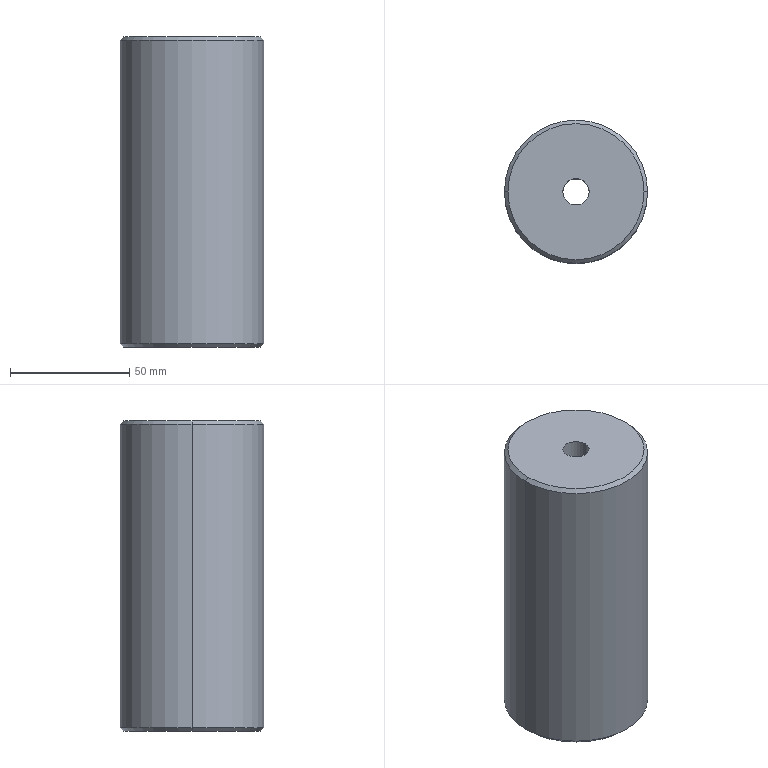Part | 1 solid | 13 faces | box 60 x 60 x 130 mm | volume 352156 mm3 | cylinder 6 | cone 4 | plane 3 | commonest cylinder face diameters 11 x2 17 x2 60 x2
STEP:
#1=CARTESIAN_POINT('',(0.,0.,0.));
#2=DIRECTION('',(0.,0.,1.));
#3=DIRECTION('',(1.,0.,0.));
#4=AXIS2_PLACEMENT_3D('',#1,#2,#3);
#5=CARTESIAN_POINT('',(24.,631.5,-191.551));
#6=VERTEX_POINT('',#5);
#7=CARTESIAN_POINT('',(24.,631.5,-64.551));
#8=VERTEX_POINT('',#7);
#9=CARTESIAN_POINT('',(24.,631.5,-191.551));
#10=DIRECTION('',(0.,0.,1.));
#11=VECTOR('',#10,1.);
#12=LINE('',#9,#11);
#13=CARTESIAN_POINT('',(-6.,631.5,-193.051));
#14=DIRECTION('',(0.,0.,1.));
#15=DIRECTION('',(0.,-1.,0.));
#16=AXIS2_PLACEMENT_3D('',#13,#14,#15);
#17=CYLINDRICAL_SURFACE('',#16,30.);
#18=CARTESIAN_POINT('',(1.571,1.5));
#19=DIRECTION('',(0.,1.));
#20=VECTOR('',#19,1.);
#21=LINE('',#18,#20);
#22=(GEOMETRIC_REPRESENTATION_CONTEXT(2)PARAMETRIC_REPRESENTATION_CONTEXT()REPRESENTATION_CONTEXT('',''));
#23=DEFINITIONAL_REPRESENTATION('',(#21),#22);
#24=PCURVE('',#17,#23);
#25=CARTESIAN_POINT('',(-6.,631.5,-193.051));
#26=DIRECTION('',(0.,0.,1.));
#27=DIRECTION('',(0.,1.,0.));
#28=AXIS2_PLACEMENT_3D('',#25,#26,#27);
#29=CYLINDRICAL_SURFACE('',#28,30.);
#30=CARTESIAN_POINT('',(4.712,1.5));
#31=DIRECTION('',(0.,1.));
#32=VECTOR('',#31,1.);
#33=LINE('',#30,#32);
#34=(GEOMETRIC_REPRESENTATION_CONTEXT(2)PARAMETRIC_REPRESENTATION_CONTEXT()REPRESENTATION_CONTEXT('',''));
#35=DEFINITIONAL_REPRESENTATION('',(#33),#34);
#36=PCURVE('',#29,#35);
#37=SURFACE_CURVE('',#12,(#24,#36),.PCURVE_S1.);
#38=EDGE_CURVE('',#6,#8,#37,.T.);
#39=ORIENTED_EDGE('',*,*,#38,.F.);
#40=CARTESIAN_POINT('',(-36.,631.5,-191.551));
#41=VERTEX_POINT('',#40);
#42=CARTESIAN_POINT('',(-6.,631.5,-191.551));
#43=DIRECTION('',(0.,0.,1.));
#44=DIRECTION('',(1.,0.,0.));
#45=AXIS2_PLACEMENT_3D('',#42,#43,#44);
#46=CIRCLE('',#45,30.);
#47=CARTESIAN_POINT('',(1.571,1.5));
#48=DIRECTION('',(1.,0.));
#49=VECTOR('',#48,1.);
#50=LINE('',#47,#49);
#51=(GEOMETRIC_REPRESENTATION_CONTEXT(2)PARAMETRIC_REPRESENTATION_CONTEXT()REPRESENTATION_CONTEXT('',''));
#52=DEFINITIONAL_REPRESENTATION('',(#50),#51);
#53=PCURVE('',#17,#52);
#54=CARTESIAN_POINT('',(-6.,631.5,-191.551));
#55=DIRECTION('',(0.,0.,1.));
#56=DIRECTION('',(0.,-1.,0.));
#57=AXIS2_PLACEMENT_3D('',#54,#55,#56);
#58=CONICAL_SURFACE('',#57,30.,0.7854);
#59=CARTESIAN_POINT('',(1.571,0.));
#60=DIRECTION('',(1.,0.));
#61=VECTOR('',#60,1.);
#62=LINE('',#59,#61);
#63=(GEOMETRIC_REPRESENTATION_CONTEXT(2)PARAMETRIC_REPRESENTATION_CONTEXT()REPRESENTATION_CONTEXT('',''));
#64=DEFINITIONAL_REPRESENTATION('',(#62),#63);
#65=PCURVE('',#58,#64);
#66=SURFACE_CURVE('',#46,(#53,#65),.PCURVE_S1.);
#67=EDGE_CURVE('',#6,#41,#66,.T.);
#68=ORIENTED_EDGE('',*,*,#67,.T.);
#69=CARTESIAN_POINT('',(-36.,631.5,-64.551));
#70=VERTEX_POINT('',#69);
#71=CARTESIAN_POINT('',(-36.,631.5,-191.551));
#72=DIRECTION('',(0.,0.,1.));
#73=VECTOR('',#72,1.);
#74=LINE('',#71,#73);
#75=CARTESIAN_POINT('',(4.712,1.5));
#76=DIRECTION('',(0.,1.));
#77=VECTOR('',#76,1.);
#78=LINE('',#75,#77);
#79=(GEOMETRIC_REPRESENTATION_CONTEXT(2)PARAMETRIC_REPRESENTATION_CONTEXT()REPRESENTATION_CONTEXT('',''));
#80=DEFINITIONAL_REPRESENTATION('',(#78),#79);
#81=PCURVE('',#17,#80);
#82=CARTESIAN_POINT('',(1.571,1.5));
#83=DIRECTION('',(0.,1.));
#84=VECTOR('',#83,1.);
#85=LINE('',#82,#84);
#86=(GEOMETRIC_REPRESENTATION_CONTEXT(2)PARAMETRIC_REPRESENTATION_CONTEXT()REPRESENTATION_CONTEXT('',''));
#87=DEFINITIONAL_REPRESENTATION('',(#85),#86);
#88=PCURVE('',#29,#87);
#89=SURFACE_CURVE('',#74,(#81,#88),.PCURVE_S1.);
#90=EDGE_CURVE('',#41,#70,#89,.T.);
#91=ORIENTED_EDGE('',*,*,#90,.T.);
#92=CARTESIAN_POINT('',(-6.,631.5,-64.551));
#93=DIRECTION('',(0.,0.,-1.));
#94=DIRECTION('',(-1.,0.,0.));
#95=AXIS2_PLACEMENT_3D('',#92,#93,#94);
#96=CIRCLE('',#95,30.);
#97=CARTESIAN_POINT('',(4.712,128.5));
#98=DIRECTION('',(-1.,0.));
#99=VECTOR('',#98,1.);
#100=LINE('',#97,#99);
#101=(GEOMETRIC_REPRESENTATION_CONTEXT(2)PARAMETRIC_REPRESENTATION_CONTEXT()REPRESENTATION_CONTEXT('',''));
#102=DEFINITIONAL_REPRESENTATION('',(#100),#101);
#103=PCURVE('',#17,#102);
#104=CARTESIAN_POINT('',(-6.,631.5,-63.051));
#105=DIRECTION('',(0.,0.,-1.));
#106=DIRECTION('',(0.,-1.,0.));
#107=AXIS2_PLACEMENT_3D('',#104,#105,#106);
#108=CONICAL_SURFACE('',#107,28.5,0.7854);
#109=CARTESIAN_POINT('',(1.571,1.5));
#110=DIRECTION('',(1.,0.));
#111=VECTOR('',#110,1.);
#112=LINE('',#109,#111);
#113=(GEOMETRIC_REPRESENTATION_CONTEXT(2)PARAMETRIC_REPRESENTATION_CONTEXT()REPRESENTATION_CONTEXT('',''));
#114=DEFINITIONAL_REPRESENTATION('',(#112),#113);
#115=PCURVE('',#108,#114);
#116=SURFACE_CURVE('',#96,(#103,#115),.PCURVE_S1.);
#117=EDGE_CURVE('',#70,#8,#116,.T.);
#118=ORIENTED_EDGE('',*,*,#117,.T.);
#119=EDGE_LOOP('',(#39,#68,#91,#118));
#120=FACE_BOUND('',#119,.T.);
#121=ADVANCED_FACE('',(#120),#17,.T.);
#122=CARTESIAN_POINT('',(-34.5,631.5,-193.051));
#123=VERTEX_POINT('',#122);
#124=CARTESIAN_POINT('',(-34.5,631.5,-193.051));
#125=DIRECTION('',(-0.7071,0.,0.7071));
#126=VECTOR('',#125,1.);
#127=LINE('',#124,#126);
#128=CARTESIAN_POINT('',(-6.,631.5,-191.551));
#129=DIRECTION('',(0.,0.,1.));
#130=DIRECTION('',(0.,1.,0.));
#131=AXIS2_PLACEMENT_3D('',#128,#129,#130);
#132=CONICAL_SURFACE('',#131,30.,0.7854);
#133=CARTESIAN_POINT('',(1.571,-1.5));
#134=DIRECTION('',(0.,1.));
#135=VECTOR('',#134,1.);
#136=LINE('',#133,#135);
#137=(GEOMETRIC_REPRESENTATION_CONTEXT(2)PARAMETRIC_REPRESENTATION_CONTEXT()REPRESENTATION_CONTEXT('',''));
#138=DEFINITIONAL_REPRESENTATION('',(#136),#137);
#139=PCURVE('',#132,#138);
#140=CARTESIAN_POINT('',(4.712,-1.5));
#141=DIRECTION('',(0.,1.));
#142=VECTOR('',#141,1.);
#143=LINE('',#140,#142);
#144=(GEOMETRIC_REPRESENTATION_CONTEXT(2)PARAMETRIC_REPRESENTATION_CONTEXT()REPRESENTATION_CONTEXT('',''));
#145=DEFINITIONAL_REPRESENTATION('',(#143),#144);
#146=PCURVE('',#58,#145);
#147=SURFACE_CURVE('',#127,(#139,#146),.PCURVE_S1.);
#148=EDGE_CURVE('',#123,#41,#147,.T.);
#149=ORIENTED_EDGE('',*,*,#148,.F.);
#150=CARTESIAN_POINT('',(22.5,631.5,-193.051));
#151=VERTEX_POINT('',#150);
#152=CARTESIAN_POINT('',(-6.,631.5,-193.051));
#153=DIRECTION('',(0.,0.,-1.));
#154=DIRECTION('',(1.,0.,0.));
#155=AXIS2_PLACEMENT_3D('',#152,#153,#154);
#156=CIRCLE('',#155,28.5);
#157=CARTESIAN_POINT('',(4.712,-1.5));
#158=DIRECTION('',(-1.,0.));
#159=VECTOR('',#158,1.);
#160=LINE('',#157,#159);
#161=(GEOMETRIC_REPRESENTATION_CONTEXT(2)PARAMETRIC_REPRESENTATION_CONTEXT()REPRESENTATION_CONTEXT('',''));
#162=DEFINITIONAL_REPRESENTATION('',(#160),#161);
#163=PCURVE('',#132,#162);
#164=CARTESIAN_POINT('',(-6.,631.5,-193.051));
#165=DIRECTION('',(0.,0.,1.));
#166=DIRECTION('',(-1.,0.,0.));
#167=AXIS2_PLACEMENT_3D('',#164,#165,#166);
#168=PLANE('',#167);
#169=CARTESIAN_POINT('',(-28.5,0.));
#170=CARTESIAN_POINT('',(-28.5,49.363));
#171=CARTESIAN_POINT('',(14.25,24.682));
#172=CARTESIAN_POINT('',(57.,0.));
#173=CARTESIAN_POINT('',(14.25,-24.682));
#174=CARTESIAN_POINT('',(-28.5,-49.363));
#175=CARTESIAN_POINT('',(-28.5,0.));
#176=(BOUNDED_CURVE()B_SPLINE_CURVE(2,(#169,#170,#171,#172,#173,#174,#175),.UNSPECIFIED.,.T.,.F.)B_SPLINE_CURVE_WITH_KNOTS((1,2,2,2,2,1),(-2.094,0.,2.094,4.189,6.283,8.378),.UNSPECIFIED.)CURVE()GEOMETRIC_REPRESENTATION_ITEM()RATIONAL_B_SPLINE_CURVE((1.,0.5,1.,0.5,1.,0.5,1.))REPRESENTATION_ITEM(''));
#177=(GEOMETRIC_REPRESENTATION_CONTEXT(2)PARAMETRIC_REPRESENTATION_CONTEXT()REPRESENTATION_CONTEXT('',''));
#178=DEFINITIONAL_REPRESENTATION('',(#176),#177);
#179=PCURVE('',#168,#178);
#180=SURFACE_CURVE('',#156,(#163,#179),.PCURVE_S1.);
#181=EDGE_CURVE('',#151,#123,#180,.T.);
#182=ORIENTED_EDGE('',*,*,#181,.F.);
#183=CARTESIAN_POINT('',(22.5,631.5,-193.051));
#184=DIRECTION('',(0.7071,0.,0.7071));
#185=VECTOR('',#184,1.);
#186=LINE('',#183,#185);
#187=CARTESIAN_POINT('',(4.712,-1.5));
#188=DIRECTION('',(0.,1.));
#189=VECTOR('',#188,1.);
#190=LINE('',#187,#189);
#191=(GEOMETRIC_REPRESENTATION_CONTEXT(2)PARAMETRIC_REPRESENTATION_CONTEXT()REPRESENTATION_CONTEXT('',''));
#192=DEFINITIONAL_REPRESENTATION('',(#190),#191);
#193=PCURVE('',#132,#192);
#194=CARTESIAN_POINT('',(1.571,-1.5));
#195=DIRECTION('',(0.,1.));
#196=VECTOR('',#195,1.);
#197=LINE('',#194,#196);
#198=(GEOMETRIC_REPRESENTATION_CONTEXT(2)PARAMETRIC_REPRESENTATION_CONTEXT()REPRESENTATION_CONTEXT('',''));
#199=DEFINITIONAL_REPRESENTATION('',(#197),#198);
#200=PCURVE('',#58,#199);
#201=SURFACE_CURVE('',#186,(#193,#200),.PCURVE_S1.);
#202=EDGE_CURVE('',#151,#6,#201,.T.);
#203=ORIENTED_EDGE('',*,*,#202,.T.);
#204=CARTESIAN_POINT('',(-6.,631.5,-191.551));
#205=DIRECTION('',(0.,0.,1.));
#206=DIRECTION('',(1.,0.,0.));
#207=AXIS2_PLACEMENT_3D('',#204,#205,#206);
#208=CIRCLE('',#207,30.);
#209=CARTESIAN_POINT('',(-1.571,0.));
#210=DIRECTION('',(1.,0.));
#211=VECTOR('',#210,1.);
#212=LINE('',#209,#211);
#213=(GEOMETRIC_REPRESENTATION_CONTEXT(2)PARAMETRIC_REPRESENTATION_CONTEXT()REPRESENTATION_CONTEXT('',''));
#214=DEFINITIONAL_REPRESENTATION('',(#212),#213);
#215=PCURVE('',#132,#214);
#216=CARTESIAN_POINT('',(-1.571,1.5));
#217=DIRECTION('',(1.,0.));
#218=VECTOR('',#217,1.);
#219=LINE('',#216,#218);
#220=(GEOMETRIC_REPRESENTATION_CONTEXT(2)PARAMETRIC_REPRESENTATION_CONTEXT()REPRESENTATION_CONTEXT('',''));
#221=DEFINITIONAL_REPRESENTATION('',(#219),#220);
#222=PCURVE('',#29,#221);
#223=SURFACE_CURVE('',#208,(#215,#222),.PCURVE_S1.);
#224=EDGE_CURVE('',#41,#6,#223,.T.);
#225=ORIENTED_EDGE('',*,*,#224,.F.);
#226=EDGE_LOOP('',(#149,#182,#203,#225));
#227=FACE_BOUND('',#226,.T.);
#228=ADVANCED_FACE('',(#227),#132,.T.);
#229=CARTESIAN_POINT('',(-14.5,631.5,-193.051));
#230=VERTEX_POINT('',#229);
#231=CARTESIAN_POINT('',(2.5,631.5,-193.051));
#232=VERTEX_POINT('',#231);
#233=CARTESIAN_POINT('',(-6.,631.5,-193.051));
#234=DIRECTION('',(0.,0.,1.));
#235=DIRECTION('',(-1.,0.,0.));
#236=AXIS2_PLACEMENT_3D('',#233,#234,#235);
#237=CIRCLE('',#236,8.5);
#238=CARTESIAN_POINT('',(0.,0.));
#239=DIRECTION('',(1.,0.));
#240=AXIS2_PLACEMENT_2D('',#238,#239);
#241=CIRCLE('',#240,8.5);
#242=(GEOMETRIC_REPRESENTATION_CONTEXT(2)PARAMETRIC_REPRESENTATION_CONTEXT()REPRESENTATION_CONTEXT('',''));
#243=DEFINITIONAL_REPRESENTATION('',(#241),#242);
#244=PCURVE('',#168,#243);
#245=CARTESIAN_POINT('',(-6.,631.5,-193.051));
#246=DIRECTION('',(0.,0.,1.));
#247=DIRECTION('',(0.,1.,0.));
#248=AXIS2_PLACEMENT_3D('',#245,#246,#247);
#249=CYLINDRICAL_SURFACE('',#248,8.5);
#250=CARTESIAN_POINT('',(1.571,0.));
#251=DIRECTION('',(1.,0.));
#252=VECTOR('',#251,1.);
#253=LINE('',#250,#252);
#254=(GEOMETRIC_REPRESENTATION_CONTEXT(2)PARAMETRIC_REPRESENTATION_CONTEXT()REPRESENTATION_CONTEXT('',''));
#255=DEFINITIONAL_REPRESENTATION('',(#253),#254);
#256=PCURVE('',#249,#255);
#257=SURFACE_CURVE('',#237,(#244,#256),.PCURVE_S1.);
#258=EDGE_CURVE('',#230,#232,#257,.T.);
#259=ORIENTED_EDGE('',*,*,#258,.T.);
#260=CARTESIAN_POINT('',(-6.,631.5,-193.051));
#261=DIRECTION('',(0.,0.,1.));
#262=DIRECTION('',(-1.,0.,0.));
#263=AXIS2_PLACEMENT_3D('',#260,#261,#262);
#264=CIRCLE('',#263,8.5);
#265=CARTESIAN_POINT('',(0.,0.));
#266=DIRECTION('',(1.,0.));
#267=AXIS2_PLACEMENT_2D('',#265,#266);
#268=CIRCLE('',#267,8.5);
#269=(GEOMETRIC_REPRESENTATION_CONTEXT(2)PARAMETRIC_REPRESENTATION_CONTEXT()REPRESENTATION_CONTEXT('',''));
#270=DEFINITIONAL_REPRESENTATION('',(#268),#269);
#271=PCURVE('',#168,#270);
#272=CARTESIAN_POINT('',(-6.,631.5,-193.051));
#273=DIRECTION('',(0.,0.,1.));
#274=DIRECTION('',(0.,-1.,0.));
#275=AXIS2_PLACEMENT_3D('',#272,#273,#274);
#276=CYLINDRICAL_SURFACE('',#275,8.5);
#277=CARTESIAN_POINT('',(-1.571,0.));
#278=DIRECTION('',(1.,0.));
#279=VECTOR('',#278,1.);
#280=LINE('',#277,#279);
#281=(GEOMETRIC_REPRESENTATION_CONTEXT(2)PARAMETRIC_REPRESENTATION_CONTEXT()REPRESENTATION_CONTEXT('',''));
#282=DEFINITIONAL_REPRESENTATION('',(#280),#281);
#283=PCURVE('',#276,#282);
#284=SURFACE_CURVE('',#264,(#271,#283),.PCURVE_S1.);
#285=EDGE_CURVE('',#232,#230,#284,.T.);
#286=ORIENTED_EDGE('',*,*,#285,.T.);
#287=EDGE_LOOP('',(#259,#286));
#288=FACE_BOUND('',#287,.T.);
#289=ORIENTED_EDGE('',*,*,#181,.T.);
#290=CARTESIAN_POINT('',(-6.,631.5,-193.051));
#291=DIRECTION('',(0.,0.,-1.));
#292=DIRECTION('',(1.,0.,0.));
#293=AXIS2_PLACEMENT_3D('',#290,#291,#292);
#294=CIRCLE('',#293,28.5);
#295=CARTESIAN_POINT('',(-28.5,0.));
#296=CARTESIAN_POINT('',(-28.5,49.363));
#297=CARTESIAN_POINT('',(14.25,24.682));
#298=CARTESIAN_POINT('',(57.,0.));
#299=CARTESIAN_POINT('',(14.25,-24.682));
#300=CARTESIAN_POINT('',(-28.5,-49.363));
#301=CARTESIAN_POINT('',(-28.5,0.));
#302=(BOUNDED_CURVE()B_SPLINE_CURVE(2,(#295,#296,#297,#298,#299,#300,#301),.UNSPECIFIED.,.T.,.F.)B_SPLINE_CURVE_WITH_KNOTS((1,2,2,2,2,1),(-2.094,0.,2.094,4.189,6.283,8.378),.UNSPECIFIED.)CURVE()GEOMETRIC_REPRESENTATION_ITEM()RATIONAL_B_SPLINE_CURVE((1.,0.5,1.,0.5,1.,0.5,1.))REPRESENTATION_ITEM(''));
#303=(GEOMETRIC_REPRESENTATION_CONTEXT(2)PARAMETRIC_REPRESENTATION_CONTEXT()REPRESENTATION_CONTEXT('',''));
#304=DEFINITIONAL_REPRESENTATION('',(#302),#303);
#305=PCURVE('',#168,#304);
#306=CARTESIAN_POINT('',(7.854,-1.5));
#307=DIRECTION('',(-1.,0.));
#308=VECTOR('',#307,1.);
#309=LINE('',#306,#308);
#310=(GEOMETRIC_REPRESENTATION_CONTEXT(2)PARAMETRIC_REPRESENTATION_CONTEXT()REPRESENTATION_CONTEXT('',''));
#311=DEFINITIONAL_REPRESENTATION('',(#309),#310);
#312=PCURVE('',#58,#311);
#313=SURFACE_CURVE('',#294,(#305,#312),.PCURVE_S1.);
#314=EDGE_CURVE('',#123,#151,#313,.T.);
#315=ORIENTED_EDGE('',*,*,#314,.T.);
#316=EDGE_LOOP('',(#289,#315));
#317=FACE_BOUND('',#316,.T.);
#318=ADVANCED_FACE('',(#288,#317),#168,.F.);
#319=ORIENTED_EDGE('',*,*,#285,.T.);
#320=CARTESIAN_POINT('',(-14.5,631.5,-173.051));
#321=VERTEX_POINT('',#320);
#322=CARTESIAN_POINT('',(-14.5,631.5,-193.051));
#323=DIRECTION('',(0.,0.,1.));
#324=VECTOR('',#323,1.);
#325=LINE('',#322,#324);
#326=CARTESIAN_POINT('',(4.712,0.));
#327=DIRECTION('',(0.,1.));
#328=VECTOR('',#327,1.);
#329=LINE('',#326,#328);
#330=(GEOMETRIC_REPRESENTATION_CONTEXT(2)PARAMETRIC_REPRESENTATION_CONTEXT()REPRESENTATION_CONTEXT('',''));
#331=DEFINITIONAL_REPRESENTATION('',(#329),#330);
#332=PCURVE('',#276,#331);
#333=CARTESIAN_POINT('',(1.571,0.));
#334=DIRECTION('',(0.,1.));
#335=VECTOR('',#334,1.);
#336=LINE('',#333,#335);
#337=(GEOMETRIC_REPRESENTATION_CONTEXT(2)PARAMETRIC_REPRESENTATION_CONTEXT()REPRESENTATION_CONTEXT('',''));
#338=DEFINITIONAL_REPRESENTATION('',(#336),#337);
#339=PCURVE('',#249,#338);
#340=SURFACE_CURVE('',#325,(#332,#339),.PCURVE_S1.);
#341=EDGE_CURVE('',#230,#321,#340,.T.);
#342=ORIENTED_EDGE('',*,*,#341,.T.);
#343=CARTESIAN_POINT('',(2.5,631.5,-173.051));
#344=VERTEX_POINT('',#343);
#345=CARTESIAN_POINT('',(-6.,631.5,-173.051));
#346=DIRECTION('',(0.,0.,1.));
#347=DIRECTION('',(-1.,0.,0.));
#348=AXIS2_PLACEMENT_3D('',#345,#346,#347);
#349=CIRCLE('',#348,8.5);
#350=CARTESIAN_POINT('',(-1.571,20.));
#351=DIRECTION('',(1.,0.));
#352=VECTOR('',#351,1.);
#353=LINE('',#350,#352);
#354=(GEOMETRIC_REPRESENTATION_CONTEXT(2)PARAMETRIC_REPRESENTATION_CONTEXT()REPRESENTATION_CONTEXT('',''));
#355=DEFINITIONAL_REPRESENTATION('',(#353),#354);
#356=PCURVE('',#276,#355);
#357=CARTESIAN_POINT('',(-6.,631.5,-173.051));
#358=DIRECTION('',(0.,0.,1.));
#359=DIRECTION('',(-1.,0.,0.));
#360=AXIS2_PLACEMENT_3D('',#357,#358,#359);
#361=PLANE('',#360);
#362=CARTESIAN_POINT('',(0.,0.));
#363=DIRECTION('',(1.,0.));
#364=AXIS2_PLACEMENT_2D('',#362,#363);
#365=CIRCLE('',#364,8.5);
#366=(GEOMETRIC_REPRESENTATION_CONTEXT(2)PARAMETRIC_REPRESENTATION_CONTEXT()REPRESENTATION_CONTEXT('',''));
#367=DEFINITIONAL_REPRESENTATION('',(#365),#366);
#368=PCURVE('',#361,#367);
#369=SURFACE_CURVE('',#349,(#356,#368),.PCURVE_S1.);
#370=EDGE_CURVE('',#344,#321,#369,.T.);
#371=ORIENTED_EDGE('',*,*,#370,.F.);
#372=CARTESIAN_POINT('',(2.5,631.5,-193.051));
#373=DIRECTION('',(0.,0.,1.));
#374=VECTOR('',#373,1.);
#375=LINE('',#372,#374);
#376=CARTESIAN_POINT('',(1.571,0.));
#377=DIRECTION('',(0.,1.));
#378=VECTOR('',#377,1.);
#379=LINE('',#376,#378);
#380=(GEOMETRIC_REPRESENTATION_CONTEXT(2)PARAMETRIC_REPRESENTATION_CONTEXT()REPRESENTATION_CONTEXT('',''));
#381=DEFINITIONAL_REPRESENTATION('',(#379),#380);
#382=PCURVE('',#276,#381);
#383=CARTESIAN_POINT('',(4.712,0.));
#384=DIRECTION('',(0.,1.));
#385=VECTOR('',#384,1.);
#386=LINE('',#383,#385);
#387=(GEOMETRIC_REPRESENTATION_CONTEXT(2)PARAMETRIC_REPRESENTATION_CONTEXT()REPRESENTATION_CONTEXT('',''));
#388=DEFINITIONAL_REPRESENTATION('',(#386),#387);
#389=PCURVE('',#249,#388);
#390=SURFACE_CURVE('',#375,(#382,#389),.PCURVE_S1.);
#391=EDGE_CURVE('',#232,#344,#390,.T.);
#392=ORIENTED_EDGE('',*,*,#391,.F.);
#393=EDGE_LOOP('',(#319,#342,#371,#392));
#394=FACE_BOUND('',#393,.F.);
#395=ADVANCED_FACE('',(#394),#276,.F.);
#396=CARTESIAN_POINT('',(-11.5,631.5,-173.051));
#397=VERTEX_POINT('',#396);
#398=CARTESIAN_POINT('',(-0.5,631.5,-173.051));
#399=VERTEX_POINT('',#398);
#400=CARTESIAN_POINT('',(-6.,631.5,-173.051));
#401=DIRECTION('',(0.,0.,1.));
#402=DIRECTION('',(-1.,0.,0.));
#403=AXIS2_PLACEMENT_3D('',#400,#401,#402);
#404=CIRCLE('',#403,5.5);
#405=CARTESIAN_POINT('',(0.,0.));
#406=DIRECTION('',(1.,0.));
#407=AXIS2_PLACEMENT_2D('',#405,#406);
#408=CIRCLE('',#407,5.5);
#409=(GEOMETRIC_REPRESENTATION_CONTEXT(2)PARAMETRIC_REPRESENTATION_CONTEXT()REPRESENTATION_CONTEXT('',''));
#410=DEFINITIONAL_REPRESENTATION('',(#408),#409);
#411=PCURVE('',#361,#410);
#412=CARTESIAN_POINT('',(-6.,631.5,-93.051));
#413=DIRECTION('',(0.,0.,1.));
#414=DIRECTION('',(0.,1.,0.));
#415=AXIS2_PLACEMENT_3D('',#412,#413,#414);
#416=CYLINDRICAL_SURFACE('',#415,5.5);
#417=CARTESIAN_POINT('',(1.571,-80.));
#418=DIRECTION('',(1.,0.));
#419=VECTOR('',#418,1.);
#420=LINE('',#417,#419);
#421=(GEOMETRIC_REPRESENTATION_CONTEXT(2)PARAMETRIC_REPRESENTATION_CONTEXT()REPRESENTATION_CONTEXT('',''));
#422=DEFINITIONAL_REPRESENTATION('',(#420),#421);
#423=PCURVE('',#416,#422);
#424=SURFACE_CURVE('',#404,(#411,#423),.PCURVE_S1.);
#425=EDGE_CURVE('',#397,#399,#424,.T.);
#426=ORIENTED_EDGE('',*,*,#425,.T.);
#427=CARTESIAN_POINT('',(-6.,631.5,-173.051));
#428=DIRECTION('',(0.,0.,1.));
#429=DIRECTION('',(-1.,0.,0.));
#430=AXIS2_PLACEMENT_3D('',#427,#428,#429);
#431=CIRCLE('',#430,5.5);
#432=CARTESIAN_POINT('',(0.,0.));
#433=DIRECTION('',(1.,0.));
#434=AXIS2_PLACEMENT_2D('',#432,#433);
#435=CIRCLE('',#434,5.5);
#436=(GEOMETRIC_REPRESENTATION_CONTEXT(2)PARAMETRIC_REPRESENTATION_CONTEXT()REPRESENTATION_CONTEXT('',''));
#437=DEFINITIONAL_REPRESENTATION('',(#435),#436);
#438=PCURVE('',#361,#437);
#439=CARTESIAN_POINT('',(-6.,631.5,-93.051));
#440=DIRECTION('',(0.,0.,1.));
#441=DIRECTION('',(0.,-1.,0.));
#442=AXIS2_PLACEMENT_3D('',#439,#440,#441);
#443=CYLINDRICAL_SURFACE('',#442,5.5);
#444=CARTESIAN_POINT('',(-1.571,-80.));
#445=DIRECTION('',(1.,0.));
#446=VECTOR('',#445,1.);
#447=LINE('',#444,#446);
#448=(GEOMETRIC_REPRESENTATION_CONTEXT(2)PARAMETRIC_REPRESENTATION_CONTEXT()REPRESENTATION_CONTEXT('',''));
#449=DEFINITIONAL_REPRESENTATION('',(#447),#448);
#450=PCURVE('',#443,#449);
#451=SURFACE_CURVE('',#431,(#438,#450),.PCURVE_S1.);
#452=EDGE_CURVE('',#399,#397,#451,.T.);
#453=ORIENTED_EDGE('',*,*,#452,.T.);
#454=EDGE_LOOP('',(#426,#453));
#455=FACE_BOUND('',#454,.T.);
#456=ORIENTED_EDGE('',*,*,#370,.F.);
#457=CARTESIAN_POINT('',(-6.,631.5,-173.051));
#458=DIRECTION('',(0.,0.,1.));
#459=DIRECTION('',(-1.,0.,0.));
#460=AXIS2_PLACEMENT_3D('',#457,#458,#459);
#461=CIRCLE('',#460,8.5);
#462=CARTESIAN_POINT('',(0.,0.));
#463=DIRECTION('',(1.,0.));
#464=AXIS2_PLACEMENT_2D('',#462,#463);
#465=CIRCLE('',#464,8.5);
#466=(GEOMETRIC_REPRESENTATION_CONTEXT(2)PARAMETRIC_REPRESENTATION_CONTEXT()REPRESENTATION_CONTEXT('',''));
#467=DEFINITIONAL_REPRESENTATION('',(#465),#466);
#468=PCURVE('',#361,#467);
#469=CARTESIAN_POINT('',(1.571,20.));
#470=DIRECTION('',(1.,0.));
#471=VECTOR('',#470,1.);
#472=LINE('',#469,#471);
#473=(GEOMETRIC_REPRESENTATION_CONTEXT(2)PARAMETRIC_REPRESENTATION_CONTEXT()REPRESENTATION_CONTEXT('',''));
#474=DEFINITIONAL_REPRESENTATION('',(#472),#473);
#475=PCURVE('',#249,#474);
#476=SURFACE_CURVE('',#461,(#468,#475),.PCURVE_S1.);
#477=EDGE_CURVE('',#321,#344,#476,.T.);
#478=ORIENTED_EDGE('',*,*,#477,.F.);
#479=EDGE_LOOP('',(#456,#478));
#480=FACE_BOUND('',#479,.T.);
#481=ADVANCED_FACE('',(#455,#480),#361,.F.);
#482=ORIENTED_EDGE('',*,*,#452,.T.);
#483=CARTESIAN_POINT('',(-11.5,631.5,-63.051));
#484=VERTEX_POINT('',#483);
#485=CARTESIAN_POINT('',(-11.5,631.5,-173.051));
#486=DIRECTION('',(0.,0.,1.));
#487=VECTOR('',#486,1.);
#488=LINE('',#485,#487);
#489=CARTESIAN_POINT('',(4.712,-80.));
#490=DIRECTION('',(0.,1.));
#491=VECTOR('',#490,1.);
#492=LINE('',#489,#491);
#493=(GEOMETRIC_REPRESENTATION_CONTEXT(2)PARAMETRIC_REPRESENTATION_CONTEXT()REPRESENTATION_CONTEXT('',''));
#494=DEFINITIONAL_REPRESENTATION('',(#492),#493);
#495=PCURVE('',#443,#494);
#496=CARTESIAN_POINT('',(1.571,-80.));
#497=DIRECTION('',(0.,1.));
#498=VECTOR('',#497,1.);
#499=LINE('',#496,#498);
#500=(GEOMETRIC_REPRESENTATION_CONTEXT(2)PARAMETRIC_REPRESENTATION_CONTEXT()REPRESENTATION_CONTEXT('',''));
#501=DEFINITIONAL_REPRESENTATION('',(#499),#500);
#502=PCURVE('',#416,#501);
#503=SURFACE_CURVE('',#488,(#495,#502),.PCURVE_S1.);
#504=EDGE_CURVE('',#397,#484,#503,.T.);
#505=ORIENTED_EDGE('',*,*,#504,.T.);
#506=CARTESIAN_POINT('',(-0.5,631.5,-63.051));
#507=VERTEX_POINT('',#506);
#508=CARTESIAN_POINT('',(-6.,631.5,-63.051));
#509=DIRECTION('',(0.,0.,1.));
#510=DIRECTION('',(-1.,0.,0.));
#511=AXIS2_PLACEMENT_3D('',#508,#509,#510);
#512=CIRCLE('',#511,5.5);
#513=CARTESIAN_POINT('',(-1.571,30.));
#514=DIRECTION('',(1.,0.));
#515=VECTOR('',#514,1.);
#516=LINE('',#513,#515);
#517=(GEOMETRIC_REPRESENTATION_CONTEXT(2)PARAMETRIC_REPRESENTATION_CONTEXT()REPRESENTATION_CONTEXT('',''));
#518=DEFINITIONAL_REPRESENTATION('',(#516),#517);
#519=PCURVE('',#443,#518);
#520=CARTESIAN_POINT('',(-6.,631.5,-63.051));
#521=DIRECTION('',(0.,0.,1.));
#522=DIRECTION('',(-1.,0.,0.));
#523=AXIS2_PLACEMENT_3D('',#520,#521,#522);
#524=PLANE('',#523);
#525=CARTESIAN_POINT('',(0.,0.));
#526=DIRECTION('',(1.,0.));
#527=AXIS2_PLACEMENT_2D('',#525,#526);
#528=CIRCLE('',#527,5.5);
#529=(GEOMETRIC_REPRESENTATION_CONTEXT(2)PARAMETRIC_REPRESENTATION_CONTEXT()REPRESENTATION_CONTEXT('',''));
#530=DEFINITIONAL_REPRESENTATION('',(#528),#529);
#531=PCURVE('',#524,#530);
#532=SURFACE_CURVE('',#512,(#519,#531),.PCURVE_S1.);
#533=EDGE_CURVE('',#507,#484,#532,.T.);
#534=ORIENTED_EDGE('',*,*,#533,.F.);
#535=CARTESIAN_POINT('',(-0.5,631.5,-173.051));
#536=DIRECTION('',(0.,0.,1.));
#537=VECTOR('',#536,1.);
#538=LINE('',#535,#537);
#539=CARTESIAN_POINT('',(1.571,-80.));
#540=DIRECTION('',(0.,1.));
#541=VECTOR('',#540,1.);
#542=LINE('',#539,#541);
#543=(GEOMETRIC_REPRESENTATION_CONTEXT(2)PARAMETRIC_REPRESENTATION_CONTEXT()REPRESENTATION_CONTEXT('',''));
#544=DEFINITIONAL_REPRESENTATION('',(#542),#543);
#545=PCURVE('',#443,#544);
#546=CARTESIAN_POINT('',(4.712,-80.));
#547=DIRECTION('',(0.,1.));
#548=VECTOR('',#547,1.);
#549=LINE('',#546,#548);
#550=(GEOMETRIC_REPRESENTATION_CONTEXT(2)PARAMETRIC_REPRESENTATION_CONTEXT()REPRESENTATION_CONTEXT('',''));
#551=DEFINITIONAL_REPRESENTATION('',(#549),#550);
#552=PCURVE('',#416,#551);
#553=SURFACE_CURVE('',#538,(#545,#552),.PCURVE_S1.);
#554=EDGE_CURVE('',#399,#507,#553,.T.);
#555=ORIENTED_EDGE('',*,*,#554,.F.);
#556=EDGE_LOOP('',(#482,#505,#534,#555));
#557=FACE_BOUND('',#556,.F.);
#558=ADVANCED_FACE('',(#557),#443,.F.);
#559=ORIENTED_EDGE('',*,*,#533,.F.);
#560=CARTESIAN_POINT('',(-6.,631.5,-63.051));
#561=DIRECTION('',(0.,0.,1.));
#562=DIRECTION('',(-1.,0.,0.));
#563=AXIS2_PLACEMENT_3D('',#560,#561,#562);
#564=CIRCLE('',#563,5.5);
#565=CARTESIAN_POINT('',(0.,0.));
#566=DIRECTION('',(1.,0.));
#567=AXIS2_PLACEMENT_2D('',#565,#566);
#568=CIRCLE('',#567,5.5);
#569=(GEOMETRIC_REPRESENTATION_CONTEXT(2)PARAMETRIC_REPRESENTATION_CONTEXT()REPRESENTATION_CONTEXT('',''));
#570=DEFINITIONAL_REPRESENTATION('',(#568),#569);
#571=PCURVE('',#524,#570);
#572=CARTESIAN_POINT('',(1.571,30.));
#573=DIRECTION('',(1.,0.));
#574=VECTOR('',#573,1.);
#575=LINE('',#572,#574);
#576=(GEOMETRIC_REPRESENTATION_CONTEXT(2)PARAMETRIC_REPRESENTATION_CONTEXT()REPRESENTATION_CONTEXT('',''));
#577=DEFINITIONAL_REPRESENTATION('',(#575),#576);
#578=PCURVE('',#416,#577);
#579=SURFACE_CURVE('',#564,(#571,#578),.PCURVE_S1.);
#580=EDGE_CURVE('',#484,#507,#579,.T.);
#581=ORIENTED_EDGE('',*,*,#580,.F.);
#582=EDGE_LOOP('',(#559,#581));
#583=FACE_BOUND('',#582,.T.);
#584=CARTESIAN_POINT('',(22.5,631.5,-63.051));
#585=VERTEX_POINT('',#584);
#586=CARTESIAN_POINT('',(-34.5,631.5,-63.051));
#587=VERTEX_POINT('',#586);
#588=CARTESIAN_POINT('',(-6.,631.5,-63.051));
#589=DIRECTION('',(0.,0.,1.));
#590=DIRECTION('',(1.,0.,0.));
#591=AXIS2_PLACEMENT_3D('',#588,#589,#590);
#592=CIRCLE('',#591,28.5);
#593=CARTESIAN_POINT('',(0.,0.));
#594=DIRECTION('',(-1.,0.));
#595=AXIS2_PLACEMENT_2D('',#593,#594);
#596=CIRCLE('',#595,28.5);
#597=(GEOMETRIC_REPRESENTATION_CONTEXT(2)PARAMETRIC_REPRESENTATION_CONTEXT()REPRESENTATION_CONTEXT('',''));
#598=DEFINITIONAL_REPRESENTATION('',(#596),#597);
#599=PCURVE('',#524,#598);
#600=CARTESIAN_POINT('',(4.712,0.));
#601=DIRECTION('',(-1.,0.));
#602=VECTOR('',#601,1.);
#603=LINE('',#600,#602);
#604=(GEOMETRIC_REPRESENTATION_CONTEXT(2)PARAMETRIC_REPRESENTATION_CONTEXT()REPRESENTATION_CONTEXT('',''));
#605=DEFINITIONAL_REPRESENTATION('',(#603),#604);
#606=PCURVE('',#108,#605);
#607=SURFACE_CURVE('',#592,(#599,#606),.PCURVE_S1.);
#608=EDGE_CURVE('',#585,#587,#607,.T.);
#609=ORIENTED_EDGE('',*,*,#608,.T.);
#610=CARTESIAN_POINT('',(-6.,631.5,-63.051));
#611=DIRECTION('',(0.,0.,1.));
#612=DIRECTION('',(1.,0.,0.));
#613=AXIS2_PLACEMENT_3D('',#610,#611,#612);
#614=CIRCLE('',#613,28.5);
#615=CARTESIAN_POINT('',(0.,0.));
#616=DIRECTION('',(-1.,0.));
#617=AXIS2_PLACEMENT_2D('',#615,#616);
#618=CIRCLE('',#617,28.5);
#619=(GEOMETRIC_REPRESENTATION_CONTEXT(2)PARAMETRIC_REPRESENTATION_CONTEXT()REPRESENTATION_CONTEXT('',''));
#620=DEFINITIONAL_REPRESENTATION('',(#618),#619);
#621=PCURVE('',#524,#620);
#622=CARTESIAN_POINT('',(-6.,631.5,-63.051));
#623=DIRECTION('',(0.,0.,-1.));
#624=DIRECTION('',(0.,1.,0.));
#625=AXIS2_PLACEMENT_3D('',#622,#623,#624);
#626=CONICAL_SURFACE('',#625,28.5,0.7854);
#627=CARTESIAN_POINT('',(7.854,0.));
#628=DIRECTION('',(-1.,0.));
#629=VECTOR('',#628,1.);
#630=LINE('',#627,#629);
#631=(GEOMETRIC_REPRESENTATION_CONTEXT(2)PARAMETRIC_REPRESENTATION_CONTEXT()REPRESENTATION_CONTEXT('',''));
#632=DEFINITIONAL_REPRESENTATION('',(#630),#631);
#633=PCURVE('',#626,#632);
#634=SURFACE_CURVE('',#614,(#621,#633),.PCURVE_S1.);
#635=EDGE_CURVE('',#587,#585,#634,.T.);
#636=ORIENTED_EDGE('',*,*,#635,.T.);
#637=EDGE_LOOP('',(#609,#636));
#638=FACE_BOUND('',#637,.T.);
#639=ADVANCED_FACE('',(#583,#638),#524,.T.);
#640=CARTESIAN_POINT('',(-34.5,631.5,-63.051));
#641=DIRECTION('',(-0.7071,0.,-0.7071));
#642=VECTOR('',#641,1.);
#643=LINE('',#640,#642);
#644=CARTESIAN_POINT('',(1.571,0.));
#645=DIRECTION('',(0.,1.));
#646=VECTOR('',#645,1.);
#647=LINE('',#644,#646);
#648=(GEOMETRIC_REPRESENTATION_CONTEXT(2)PARAMETRIC_REPRESENTATION_CONTEXT()REPRESENTATION_CONTEXT('',''));
#649=DEFINITIONAL_REPRESENTATION('',(#647),#648);
#650=PCURVE('',#108,#649);
#651=CARTESIAN_POINT('',(4.712,0.));
#652=DIRECTION('',(0.,1.));
#653=VECTOR('',#652,1.);
#654=LINE('',#651,#653);
#655=(GEOMETRIC_REPRESENTATION_CONTEXT(2)PARAMETRIC_REPRESENTATION_CONTEXT()REPRESENTATION_CONTEXT('',''));
#656=DEFINITIONAL_REPRESENTATION('',(#654),#655);
#657=PCURVE('',#626,#656);
#658=SURFACE_CURVE('',#643,(#650,#657),.PCURVE_S1.);
#659=EDGE_CURVE('',#587,#70,#658,.T.);
#660=ORIENTED_EDGE('',*,*,#659,.F.);
#661=ORIENTED_EDGE('',*,*,#608,.F.);
#662=CARTESIAN_POINT('',(22.5,631.5,-63.051));
#663=DIRECTION('',(0.7071,0.,-0.7071));
#664=VECTOR('',#663,1.);
#665=LINE('',#662,#664);
#666=CARTESIAN_POINT('',(4.712,0.));
#667=DIRECTION('',(0.,1.));
#668=VECTOR('',#667,1.);
#669=LINE('',#666,#668);
#670=(GEOMETRIC_REPRESENTATION_CONTEXT(2)PARAMETRIC_REPRESENTATION_CONTEXT()REPRESENTATION_CONTEXT('',''));
#671=DEFINITIONAL_REPRESENTATION('',(#669),#670);
#672=PCURVE('',#108,#671);
#673=CARTESIAN_POINT('',(1.571,0.));
#674=DIRECTION('',(0.,1.));
#675=VECTOR('',#674,1.);
#676=LINE('',#673,#675);
#677=(GEOMETRIC_REPRESENTATION_CONTEXT(2)PARAMETRIC_REPRESENTATION_CONTEXT()REPRESENTATION_CONTEXT('',''));
#678=DEFINITIONAL_REPRESENTATION('',(#676),#677);
#679=PCURVE('',#626,#678);
#680=SURFACE_CURVE('',#665,(#672,#679),.PCURVE_S1.);
#681=EDGE_CURVE('',#585,#8,#680,.T.);
#682=ORIENTED_EDGE('',*,*,#681,.T.);
#683=ORIENTED_EDGE('',*,*,#117,.F.);
#684=EDGE_LOOP('',(#660,#661,#682,#683));
#685=FACE_BOUND('',#684,.T.);
#686=ADVANCED_FACE('',(#685),#108,.T.);
#687=ORIENTED_EDGE('',*,*,#38,.T.);
#688=CARTESIAN_POINT('',(-6.,631.5,-64.551));
#689=DIRECTION('',(0.,0.,-1.));
#690=DIRECTION('',(-1.,0.,0.));
#691=AXIS2_PLACEMENT_3D('',#688,#689,#690);
#692=CIRCLE('',#691,30.);
#693=CARTESIAN_POINT('',(7.854,128.5));
#694=DIRECTION('',(-1.,0.));
#695=VECTOR('',#694,1.);
#696=LINE('',#693,#695);
#697=(GEOMETRIC_REPRESENTATION_CONTEXT(2)PARAMETRIC_REPRESENTATION_CONTEXT()REPRESENTATION_CONTEXT('',''));
#698=DEFINITIONAL_REPRESENTATION('',(#696),#697);
#699=PCURVE('',#29,#698);
#700=CARTESIAN_POINT('',(-1.571,1.5));
#701=DIRECTION('',(1.,0.));
#702=VECTOR('',#701,1.);
#703=LINE('',#700,#702);
#704=(GEOMETRIC_REPRESENTATION_CONTEXT(2)PARAMETRIC_REPRESENTATION_CONTEXT()REPRESENTATION_CONTEXT('',''));
#705=DEFINITIONAL_REPRESENTATION('',(#703),#704);
#706=PCURVE('',#626,#705);
#707=SURFACE_CURVE('',#692,(#699,#706),.PCURVE_S1.);
#708=EDGE_CURVE('',#8,#70,#707,.T.);
#709=ORIENTED_EDGE('',*,*,#708,.T.);
#710=ORIENTED_EDGE('',*,*,#90,.F.);
#711=ORIENTED_EDGE('',*,*,#224,.T.);
#712=EDGE_LOOP('',(#687,#709,#710,#711));
#713=FACE_BOUND('',#712,.T.);
#714=ADVANCED_FACE('',(#713),#29,.T.);
#715=ORIENTED_EDGE('',*,*,#148,.T.);
#716=ORIENTED_EDGE('',*,*,#67,.F.);
#717=ORIENTED_EDGE('',*,*,#202,.F.);
#718=ORIENTED_EDGE('',*,*,#314,.F.);
#719=EDGE_LOOP('',(#715,#716,#717,#718));
#720=FACE_BOUND('',#719,.T.);
#721=ADVANCED_FACE('',(#720),#58,.T.);
#722=ORIENTED_EDGE('',*,*,#477,.F.);
#723=ORIENTED_EDGE('',*,*,#341,.F.);
#724=ORIENTED_EDGE('',*,*,#258,.T.);
#725=ORIENTED_EDGE('',*,*,#391,.T.);
#726=EDGE_LOOP('',(#722,#723,#724,#725));
#727=FACE_BOUND('',#726,.F.);
#728=ADVANCED_FACE('',(#727),#249,.F.);
#729=ORIENTED_EDGE('',*,*,#580,.F.);
#730=ORIENTED_EDGE('',*,*,#504,.F.);
#731=ORIENTED_EDGE('',*,*,#425,.T.);
#732=ORIENTED_EDGE('',*,*,#554,.T.);
#733=EDGE_LOOP('',(#729,#730,#731,#732));
#734=FACE_BOUND('',#733,.F.);
#735=ADVANCED_FACE('',(#734),#416,.F.);
#736=ORIENTED_EDGE('',*,*,#659,.T.);
#737=ORIENTED_EDGE('',*,*,#708,.F.);
#738=ORIENTED_EDGE('',*,*,#681,.F.);
#739=ORIENTED_EDGE('',*,*,#635,.F.);
#740=EDGE_LOOP('',(#736,#737,#738,#739));
#741=FACE_BOUND('',#740,.T.);
#742=ADVANCED_FACE('',(#741),#626,.T.);
#743=CLOSED_SHELL('',(#121,#228,#318,#395,#481,#558,#639,#686,#714,#721,#728,#735,#742));
#744=MANIFOLD_SOLID_BREP('',#743);
#745=(LENGTH_UNIT()NAMED_UNIT(*)SI_UNIT(.MILLI.,.METRE.));
#746=UNCERTAINTY_MEASURE_WITH_UNIT(LENGTH_MEASURE(0.0000001),#745,'','');
#747=(NAMED_UNIT(*)PLANE_ANGLE_UNIT()SI_UNIT($,.RADIAN.));
#748=(NAMED_UNIT(*)SI_UNIT($,.STERADIAN.)SOLID_ANGLE_UNIT());
#749=(GEOMETRIC_REPRESENTATION_CONTEXT(3)GLOBAL_UNCERTAINTY_ASSIGNED_CONTEXT((#746))GLOBAL_UNIT_ASSIGNED_CONTEXT((#745,#747,#748))REPRESENTATION_CONTEXT('',''));
#750=ADVANCED_BREP_SHAPE_REPRESENTATION('',(#4,#744),#749);